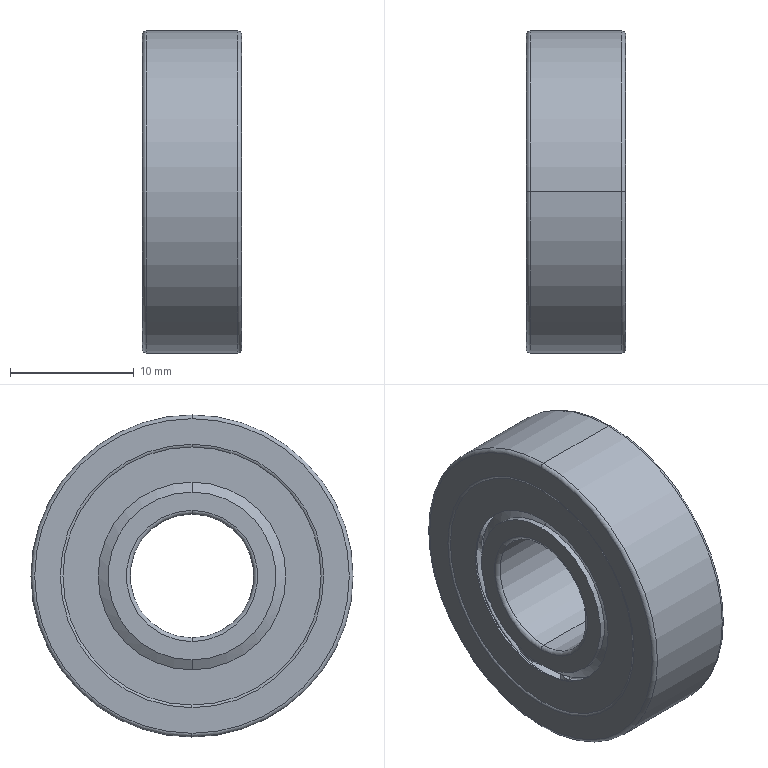Part | SolidWorks | features Revolution 5, CirPattern 2, RefAxis 1, RevCut 1 | 13 solids | 162 faces | box 8 x 26 x 26 mm | volume 2677 mm3 | cylinder 58 | sphere 48 | plane 30 | torus 22 | cone 4 | commonest cylinder face diameters 17.2 x21 18.8 x21 13.556 x4 15.333 x4 20.667 x4 10 x2